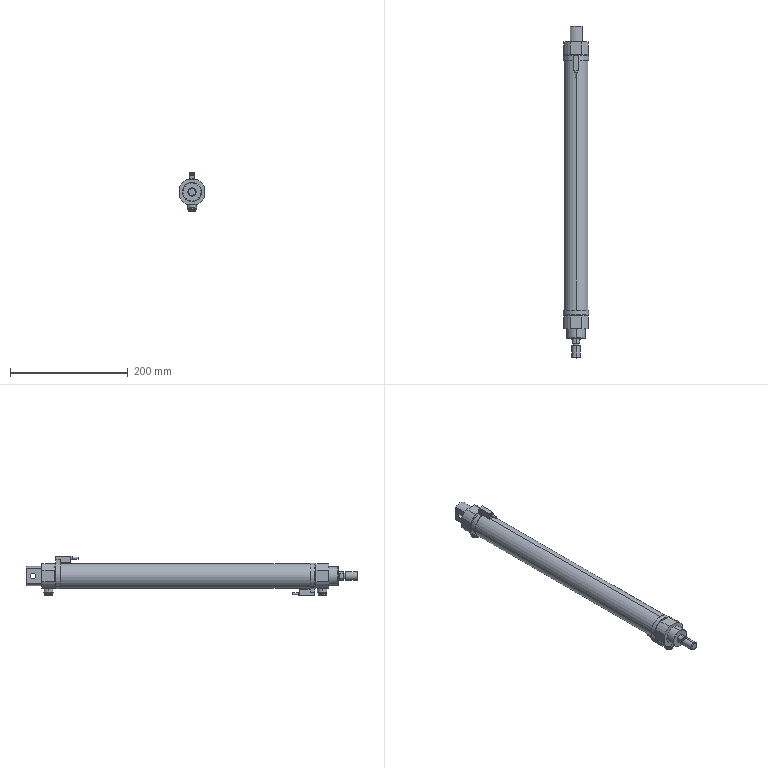Part | SolidWorks | features BaseBody 1 | 1 solid | 145 faces | box 44 x 565 x 68 mm | volume 725736 mm3 | cylinder 69 | plane 66 | cone 10 | commonest cylinder face diameters 14 x8 46.5 x8 42 x6 44 x6 3.4 x4 6 x4